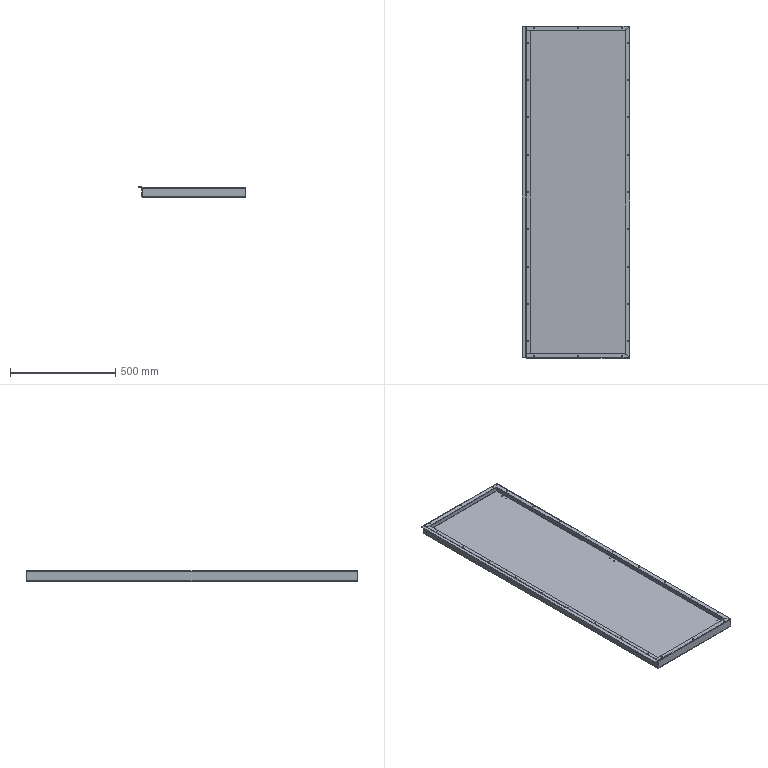Part | SolidWorks | 2 solids | 136 faces | box 512 x 1578 x 48 mm | volume 2651917 mm3 | cylinder 76 | plane 48 | spline 12 | commonest cylinder face diameters 5 x60 1.473 x8 6.473 x8